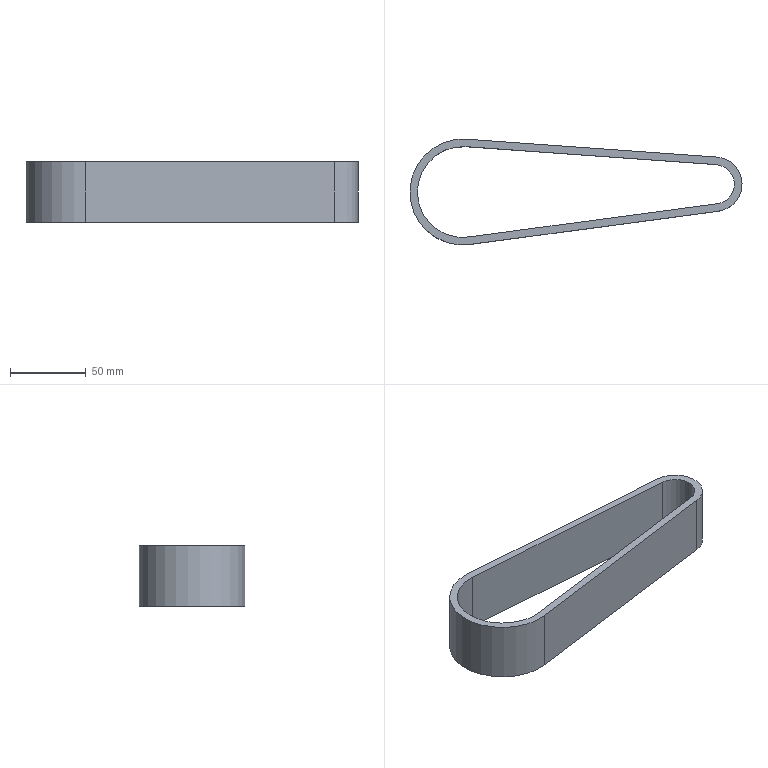Part | SolidWorks | features BaseBody 1 | 1 solid | 12 faces | box 219.551 x 70 x 40 mm | volume 97158 mm3 | cylinder 6 | plane 6 | commonest cylinder face diameters 26 x2 36 x2 60 x1 70 x1
STEP:
#1=CARTESIAN_POINT('',(-274.757,49.399,20.));
#2=VERTEX_POINT('',#1);
#3=CARTESIAN_POINT('',(-263.488,62.685,20.));
#4=VERTEX_POINT('',#3);
#5=CARTESIAN_POINT('',(-276.482,62.284,20.));
#6=DIRECTION('',(0.,0.,1.));
#7=DIRECTION('',(-0.9995,-0.03088,0.));
#8=AXIS2_PLACEMENT_3D('',#5,#6,#7);
#9=CIRCLE('',#8,13.);
#10=EDGE_CURVE('',#2,#4,#9,.T.);
#11=ORIENTED_EDGE('',*,*,#10,.T.);
#12=CARTESIAN_POINT('',(-263.488,62.685,-20.));
#13=VERTEX_POINT('',#12);
#14=CARTESIAN_POINT('',(-263.488,62.685,20.));
#15=DIRECTION('',(0.,0.,-1.));
#16=VECTOR('',#15,1000.);
#17=LINE('',#14,#16);
#18=EDGE_CURVE('',#4,#13,#17,.T.);
#19=ORIENTED_EDGE('',*,*,#18,.T.);
#20=CARTESIAN_POINT('',(-274.757,49.399,-20.));
#21=VERTEX_POINT('',#20);
#22=CARTESIAN_POINT('',(-276.482,62.284,-20.));
#23=DIRECTION('',(0.,0.,1.));
#24=DIRECTION('',(-0.9995,-0.03088,0.));
#25=AXIS2_PLACEMENT_3D('',#22,#23,#24);
#26=CIRCLE('',#25,13.);
#27=EDGE_CURVE('',#21,#13,#26,.T.);
#28=ORIENTED_EDGE('',*,*,#27,.F.);
#29=CARTESIAN_POINT('',(-274.757,49.399,20.));
#30=DIRECTION('',(0.,0.,-1.));
#31=VECTOR('',#30,1000.);
#32=LINE('',#29,#31);
#33=EDGE_CURVE('',#2,#21,#32,.T.);
#34=ORIENTED_EDGE('',*,*,#33,.F.);
#35=EDGE_LOOP('',(#11,#19,#28,#34));
#36=FACE_OUTER_BOUND('',#35,.T.);
#37=CARTESIAN_POINT('',(-276.482,62.284,20.));
#38=DIRECTION('',(0.,0.,-1.));
#39=DIRECTION('',(0.9995,0.03088,0.));
#40=AXIS2_PLACEMENT_3D('',#37,#38,#39);
#41=CYLINDRICAL_SURFACE('',#40,13.);
#42=ADVANCED_FACE('',(#36),#41,.F.);
#43=CARTESIAN_POINT('',(-258.49,62.84,20.));
#44=VERTEX_POINT('',#43);
#45=CARTESIAN_POINT('',(-275.199,80.238,20.));
#46=VERTEX_POINT('',#45);
#47=CARTESIAN_POINT('',(-276.482,62.284,20.));
#48=DIRECTION('',(0.,0.,1.));
#49=DIRECTION('',(-0.9995,-0.03088,0.));
#50=AXIS2_PLACEMENT_3D('',#47,#48,#49);
#51=CIRCLE('',#50,18.);
#52=EDGE_CURVE('',#44,#46,#51,.T.);
#53=ORIENTED_EDGE('',*,*,#52,.F.);
#54=CARTESIAN_POINT('',(-258.49,62.84,-20.));
#55=VERTEX_POINT('',#54);
#56=CARTESIAN_POINT('',(-258.49,62.84,20.));
#57=DIRECTION('',(0.,0.,-1.));
#58=VECTOR('',#57,1000.);
#59=LINE('',#56,#58);
#60=EDGE_CURVE('',#44,#55,#59,.T.);
#61=ORIENTED_EDGE('',*,*,#60,.T.);
#62=CARTESIAN_POINT('',(-275.199,80.238,-20.));
#63=VERTEX_POINT('',#62);
#64=CARTESIAN_POINT('',(-276.482,62.284,-20.));
#65=DIRECTION('',(0.,0.,1.));
#66=DIRECTION('',(-0.9995,-0.03088,0.));
#67=AXIS2_PLACEMENT_3D('',#64,#65,#66);
#68=CIRCLE('',#67,18.);
#69=EDGE_CURVE('',#55,#63,#68,.T.);
#70=ORIENTED_EDGE('',*,*,#69,.T.);
#71=CARTESIAN_POINT('',(-275.199,80.238,20.));
#72=DIRECTION('',(0.,0.,-1.));
#73=VECTOR('',#72,1000.);
#74=LINE('',#71,#73);
#75=EDGE_CURVE('',#46,#63,#74,.T.);
#76=ORIENTED_EDGE('',*,*,#75,.F.);
#77=EDGE_LOOP('',(#53,#61,#70,#76));
#78=FACE_OUTER_BOUND('',#77,.T.);
#79=CARTESIAN_POINT('',(-276.482,62.284,20.));
#80=DIRECTION('',(0.,0.,-1.));
#81=DIRECTION('',(0.9995,0.03088,0.));
#82=AXIS2_PLACEMENT_3D('',#79,#80,#81);
#83=CYLINDRICAL_SURFACE('',#82,18.);
#84=ADVANCED_FACE('',(#78),#83,.T.);
#85=CARTESIAN_POINT('',(-274.093,44.443,20.));
#86=VERTEX_POINT('',#85);
#87=CARTESIAN_POINT('',(-276.482,62.284,20.));
#88=DIRECTION('',(0.,0.,1.));
#89=DIRECTION('',(-0.9995,-0.03088,0.));
#90=AXIS2_PLACEMENT_3D('',#87,#88,#89);
#91=CIRCLE('',#90,18.);
#92=EDGE_CURVE('',#86,#44,#91,.T.);
#93=ORIENTED_EDGE('',*,*,#92,.T.);
#94=ORIENTED_EDGE('',*,*,#52,.T.);
#95=CARTESIAN_POINT('',(-440.538,92.049,20.));
#96=VERTEX_POINT('',#95);
#97=CARTESIAN_POINT('',(-275.199,80.238,20.));
#98=DIRECTION('',(-0.9975,0.07126,0.));
#99=VECTOR('',#98,1000.);
#100=LINE('',#97,#99);
#101=EDGE_CURVE('',#46,#96,#100,.T.);
#102=ORIENTED_EDGE('',*,*,#101,.T.);
#103=CARTESIAN_POINT('',(-438.388,22.448,20.));
#104=VERTEX_POINT('',#103);
#105=CARTESIAN_POINT('',(-443.032,57.138,20.));
#106=DIRECTION('',(0.,0.,1.));
#107=DIRECTION('',(-0.9995,-0.03088,0.));
#108=AXIS2_PLACEMENT_3D('',#105,#106,#107);
#109=CIRCLE('',#108,35.);
#110=EDGE_CURVE('',#96,#104,#109,.T.);
#111=ORIENTED_EDGE('',*,*,#110,.T.);
#112=CARTESIAN_POINT('',(-274.093,44.443,20.));
#113=DIRECTION('',(0.9912,0.1327,0.));
#114=VECTOR('',#113,1000.);
#115=LINE('',#112,#114);
#116=EDGE_CURVE('',#104,#86,#115,.T.);
#117=ORIENTED_EDGE('',*,*,#116,.T.);
#118=EDGE_LOOP('',(#93,#94,#102,#111,#117));
#119=FACE_OUTER_BOUND('',#118,.T.);
#120=CARTESIAN_POINT('',(-439.052,27.404,20.));
#121=VERTEX_POINT('',#120);
#122=CARTESIAN_POINT('',(-274.757,49.399,20.));
#123=DIRECTION('',(0.9912,0.1327,0.));
#124=VECTOR('',#123,1000.);
#125=LINE('',#122,#124);
#126=EDGE_CURVE('',#121,#2,#125,.T.);
#127=ORIENTED_EDGE('',*,*,#126,.F.);
#128=CARTESIAN_POINT('',(-440.895,87.062,20.));
#129=VERTEX_POINT('',#128);
#130=CARTESIAN_POINT('',(-443.032,57.138,20.));
#131=DIRECTION('',(0.,0.,1.));
#132=DIRECTION('',(-0.9995,-0.03088,0.));
#133=AXIS2_PLACEMENT_3D('',#130,#131,#132);
#134=CIRCLE('',#133,30.);
#135=EDGE_CURVE('',#129,#121,#134,.T.);
#136=ORIENTED_EDGE('',*,*,#135,.F.);
#137=CARTESIAN_POINT('',(-275.555,75.251,20.));
#138=VERTEX_POINT('',#137);
#139=CARTESIAN_POINT('',(-275.555,75.251,20.));
#140=DIRECTION('',(-0.9975,0.07126,0.));
#141=VECTOR('',#140,1000.);
#142=LINE('',#139,#141);
#143=EDGE_CURVE('',#138,#129,#142,.T.);
#144=ORIENTED_EDGE('',*,*,#143,.F.);
#145=CARTESIAN_POINT('',(-276.482,62.284,20.));
#146=DIRECTION('',(0.,0.,1.));
#147=DIRECTION('',(-0.9995,-0.03088,0.));
#148=AXIS2_PLACEMENT_3D('',#145,#146,#147);
#149=CIRCLE('',#148,13.);
#150=EDGE_CURVE('',#4,#138,#149,.T.);
#151=ORIENTED_EDGE('',*,*,#150,.F.);
#152=ORIENTED_EDGE('',*,*,#10,.F.);
#153=EDGE_LOOP('',(#127,#136,#144,#151,#152));
#154=FACE_BOUND('',#153,.T.);
#155=CARTESIAN_POINT('',(-276.482,62.284,20.));
#156=DIRECTION('',(0.,0.,1.));
#157=DIRECTION('',(-0.9995,-0.03088,0.));
#158=AXIS2_PLACEMENT_3D('',#155,#156,#157);
#159=PLANE('',#158);
#160=ADVANCED_FACE('',(#119,#154),#159,.T.);
#161=CARTESIAN_POINT('',(-274.093,44.443,-20.));
#162=VERTEX_POINT('',#161);
#163=CARTESIAN_POINT('',(-276.482,62.284,-20.));
#164=DIRECTION('',(0.,0.,1.));
#165=DIRECTION('',(-0.9995,-0.03088,0.));
#166=AXIS2_PLACEMENT_3D('',#163,#164,#165);
#167=CIRCLE('',#166,18.);
#168=EDGE_CURVE('',#162,#55,#167,.T.);
#169=ORIENTED_EDGE('',*,*,#168,.F.);
#170=CARTESIAN_POINT('',(-438.388,22.448,-20.));
#171=VERTEX_POINT('',#170);
#172=CARTESIAN_POINT('',(-274.093,44.443,-20.));
#173=DIRECTION('',(0.9912,0.1327,0.));
#174=VECTOR('',#173,1000.);
#175=LINE('',#172,#174);
#176=EDGE_CURVE('',#171,#162,#175,.T.);
#177=ORIENTED_EDGE('',*,*,#176,.F.);
#178=CARTESIAN_POINT('',(-440.538,92.049,-20.));
#179=VERTEX_POINT('',#178);
#180=CARTESIAN_POINT('',(-443.032,57.138,-20.));
#181=DIRECTION('',(0.,0.,1.));
#182=DIRECTION('',(-0.9995,-0.03088,0.));
#183=AXIS2_PLACEMENT_3D('',#180,#181,#182);
#184=CIRCLE('',#183,35.);
#185=EDGE_CURVE('',#179,#171,#184,.T.);
#186=ORIENTED_EDGE('',*,*,#185,.F.);
#187=CARTESIAN_POINT('',(-275.199,80.238,-20.));
#188=DIRECTION('',(-0.9975,0.07126,0.));
#189=VECTOR('',#188,1000.);
#190=LINE('',#187,#189);
#191=EDGE_CURVE('',#63,#179,#190,.T.);
#192=ORIENTED_EDGE('',*,*,#191,.F.);
#193=ORIENTED_EDGE('',*,*,#69,.F.);
#194=EDGE_LOOP('',(#169,#177,#186,#192,#193));
#195=FACE_OUTER_BOUND('',#194,.T.);
#196=CARTESIAN_POINT('',(-440.895,87.062,-20.));
#197=VERTEX_POINT('',#196);
#198=CARTESIAN_POINT('',(-439.052,27.404,-20.));
#199=VERTEX_POINT('',#198);
#200=CARTESIAN_POINT('',(-443.032,57.138,-20.));
#201=DIRECTION('',(0.,0.,1.));
#202=DIRECTION('',(-0.9995,-0.03088,0.));
#203=AXIS2_PLACEMENT_3D('',#200,#201,#202);
#204=CIRCLE('',#203,30.);
#205=EDGE_CURVE('',#197,#199,#204,.T.);
#206=ORIENTED_EDGE('',*,*,#205,.T.);
#207=CARTESIAN_POINT('',(-274.757,49.399,-20.));
#208=DIRECTION('',(0.9912,0.1327,0.));
#209=VECTOR('',#208,1000.);
#210=LINE('',#207,#209);
#211=EDGE_CURVE('',#199,#21,#210,.T.);
#212=ORIENTED_EDGE('',*,*,#211,.T.);
#213=ORIENTED_EDGE('',*,*,#27,.T.);
#214=CARTESIAN_POINT('',(-275.555,75.251,-20.));
#215=VERTEX_POINT('',#214);
#216=CARTESIAN_POINT('',(-276.482,62.284,-20.));
#217=DIRECTION('',(0.,0.,1.));
#218=DIRECTION('',(-0.9995,-0.03088,0.));
#219=AXIS2_PLACEMENT_3D('',#216,#217,#218);
#220=CIRCLE('',#219,13.);
#221=EDGE_CURVE('',#13,#215,#220,.T.);
#222=ORIENTED_EDGE('',*,*,#221,.T.);
#223=CARTESIAN_POINT('',(-275.555,75.251,-20.));
#224=DIRECTION('',(-0.9975,0.07126,0.));
#225=VECTOR('',#224,1000.);
#226=LINE('',#223,#225);
#227=EDGE_CURVE('',#215,#197,#226,.T.);
#228=ORIENTED_EDGE('',*,*,#227,.T.);
#229=EDGE_LOOP('',(#206,#212,#213,#222,#228));
#230=FACE_BOUND('',#229,.T.);
#231=CARTESIAN_POINT('',(-276.482,62.284,-20.));
#232=DIRECTION('',(0.,0.,1.));
#233=DIRECTION('',(-0.9995,-0.03088,0.));
#234=AXIS2_PLACEMENT_3D('',#231,#232,#233);
#235=PLANE('',#234);
#236=ADVANCED_FACE('',(#195,#230),#235,.F.);
#237=ORIENTED_EDGE('',*,*,#60,.F.);
#238=ORIENTED_EDGE('',*,*,#92,.F.);
#239=CARTESIAN_POINT('',(-274.093,44.443,20.));
#240=DIRECTION('',(0.,0.,-1.));
#241=VECTOR('',#240,1000.);
#242=LINE('',#239,#241);
#243=EDGE_CURVE('',#86,#162,#242,.T.);
#244=ORIENTED_EDGE('',*,*,#243,.T.);
#245=ORIENTED_EDGE('',*,*,#168,.T.);
#246=EDGE_LOOP('',(#237,#238,#244,#245));
#247=FACE_OUTER_BOUND('',#246,.T.);
#248=CARTESIAN_POINT('',(-276.482,62.284,20.));
#249=DIRECTION('',(0.,0.,-1.));
#250=DIRECTION('',(0.9995,0.03088,0.));
#251=AXIS2_PLACEMENT_3D('',#248,#249,#250);
#252=CYLINDRICAL_SURFACE('',#251,18.);
#253=ADVANCED_FACE('',(#247),#252,.T.);
#254=ORIENTED_EDGE('',*,*,#191,.T.);
#255=CARTESIAN_POINT('',(-440.538,92.049,20.));
#256=DIRECTION('',(0.,0.,-1.));
#257=VECTOR('',#256,1000.);
#258=LINE('',#255,#257);
#259=EDGE_CURVE('',#96,#179,#258,.T.);
#260=ORIENTED_EDGE('',*,*,#259,.F.);
#261=ORIENTED_EDGE('',*,*,#101,.F.);
#262=ORIENTED_EDGE('',*,*,#75,.T.);
#263=EDGE_LOOP('',(#254,#260,#261,#262));
#264=FACE_OUTER_BOUND('',#263,.T.);
#265=CARTESIAN_POINT('',(-275.199,80.238,20.));
#266=DIRECTION('',(-0.07126,-0.9975,0.));
#267=DIRECTION('',(0.9975,-0.07126,0.));
#268=AXIS2_PLACEMENT_3D('',#265,#266,#267);
#269=PLANE('',#268);
#270=ADVANCED_FACE('',(#264),#269,.F.);
#271=ORIENTED_EDGE('',*,*,#185,.T.);
#272=CARTESIAN_POINT('',(-438.388,22.448,20.));
#273=DIRECTION('',(0.,0.,-1.));
#274=VECTOR('',#273,1000.);
#275=LINE('',#272,#274);
#276=EDGE_CURVE('',#104,#171,#275,.T.);
#277=ORIENTED_EDGE('',*,*,#276,.F.);
#278=ORIENTED_EDGE('',*,*,#110,.F.);
#279=ORIENTED_EDGE('',*,*,#259,.T.);
#280=EDGE_LOOP('',(#271,#277,#278,#279));
#281=FACE_OUTER_BOUND('',#280,.T.);
#282=CARTESIAN_POINT('',(-443.032,57.138,20.));
#283=DIRECTION('',(0.,0.,-1.));
#284=DIRECTION('',(0.9995,0.03088,0.));
#285=AXIS2_PLACEMENT_3D('',#282,#283,#284);
#286=CYLINDRICAL_SURFACE('',#285,35.);
#287=ADVANCED_FACE('',(#281),#286,.T.);
#288=ORIENTED_EDGE('',*,*,#176,.T.);
#289=ORIENTED_EDGE('',*,*,#243,.F.);
#290=ORIENTED_EDGE('',*,*,#116,.F.);
#291=ORIENTED_EDGE('',*,*,#276,.T.);
#292=EDGE_LOOP('',(#288,#289,#290,#291));
#293=FACE_OUTER_BOUND('',#292,.T.);
#294=CARTESIAN_POINT('',(-274.093,44.443,20.));
#295=DIRECTION('',(-0.1327,0.9912,0.));
#296=DIRECTION('',(-0.9912,-0.1327,0.));
#297=AXIS2_PLACEMENT_3D('',#294,#295,#296);
#298=PLANE('',#297);
#299=ADVANCED_FACE('',(#293),#298,.F.);
#300=ORIENTED_EDGE('',*,*,#205,.F.);
#301=CARTESIAN_POINT('',(-440.895,87.062,20.));
#302=DIRECTION('',(0.,0.,-1.));
#303=VECTOR('',#302,1000.);
#304=LINE('',#301,#303);
#305=EDGE_CURVE('',#129,#197,#304,.T.);
#306=ORIENTED_EDGE('',*,*,#305,.F.);
#307=ORIENTED_EDGE('',*,*,#135,.T.);
#308=CARTESIAN_POINT('',(-439.052,27.404,20.));
#309=DIRECTION('',(0.,0.,-1.));
#310=VECTOR('',#309,1000.);
#311=LINE('',#308,#310);
#312=EDGE_CURVE('',#121,#199,#311,.T.);
#313=ORIENTED_EDGE('',*,*,#312,.T.);
#314=EDGE_LOOP('',(#300,#306,#307,#313));
#315=FACE_OUTER_BOUND('',#314,.T.);
#316=CARTESIAN_POINT('',(-443.032,57.138,20.));
#317=DIRECTION('',(0.,0.,-1.));
#318=DIRECTION('',(0.9995,0.03088,0.));
#319=AXIS2_PLACEMENT_3D('',#316,#317,#318);
#320=CYLINDRICAL_SURFACE('',#319,30.);
#321=ADVANCED_FACE('',(#315),#320,.F.);
#322=ORIENTED_EDGE('',*,*,#211,.F.);
#323=ORIENTED_EDGE('',*,*,#312,.F.);
#324=ORIENTED_EDGE('',*,*,#126,.T.);
#325=ORIENTED_EDGE('',*,*,#33,.T.);
#326=EDGE_LOOP('',(#322,#323,#324,#325));
#327=FACE_OUTER_BOUND('',#326,.T.);
#328=CARTESIAN_POINT('',(-274.757,49.399,20.));
#329=DIRECTION('',(-0.1327,0.9912,0.));
#330=DIRECTION('',(-0.9912,-0.1327,0.));
#331=AXIS2_PLACEMENT_3D('',#328,#329,#330);
#332=PLANE('',#331);
#333=ADVANCED_FACE('',(#327),#332,.T.);
#334=ORIENTED_EDGE('',*,*,#18,.F.);
#335=ORIENTED_EDGE('',*,*,#150,.T.);
#336=CARTESIAN_POINT('',(-275.555,75.251,20.));
#337=DIRECTION('',(0.,0.,-1.));
#338=VECTOR('',#337,1000.);
#339=LINE('',#336,#338);
#340=EDGE_CURVE('',#138,#215,#339,.T.);
#341=ORIENTED_EDGE('',*,*,#340,.T.);
#342=ORIENTED_EDGE('',*,*,#221,.F.);
#343=EDGE_LOOP('',(#334,#335,#341,#342));
#344=FACE_OUTER_BOUND('',#343,.T.);
#345=CARTESIAN_POINT('',(-276.482,62.284,20.));
#346=DIRECTION('',(0.,0.,-1.));
#347=DIRECTION('',(0.9995,0.03088,0.));
#348=AXIS2_PLACEMENT_3D('',#345,#346,#347);
#349=CYLINDRICAL_SURFACE('',#348,13.);
#350=ADVANCED_FACE('',(#344),#349,.F.);
#351=ORIENTED_EDGE('',*,*,#227,.F.);
#352=ORIENTED_EDGE('',*,*,#340,.F.);
#353=ORIENTED_EDGE('',*,*,#143,.T.);
#354=ORIENTED_EDGE('',*,*,#305,.T.);
#355=EDGE_LOOP('',(#351,#352,#353,#354));
#356=FACE_OUTER_BOUND('',#355,.T.);
#357=CARTESIAN_POINT('',(-275.555,75.251,20.));
#358=DIRECTION('',(-0.07126,-0.9975,0.));
#359=DIRECTION('',(0.9975,-0.07126,0.));
#360=AXIS2_PLACEMENT_3D('',#357,#358,#359);
#361=PLANE('',#360);
#362=ADVANCED_FACE('',(#356),#361,.T.);
#363=CLOSED_SHELL('',(#42,#84,#160,#236,#253,#270,#287,#299,#321,#333,#350,#362));
#364=MANIFOLD_SOLID_BREP('',#363);
#365=CARTESIAN_POINT('',(0.,0.,0.));
#366=DIRECTION('',(0.,0.,1.));
#367=DIRECTION('',(1.,0.,0.));
#368=AXIS2_PLACEMENT_3D('',#365,#366,#367);
#369=(LENGTH_UNIT()NAMED_UNIT(*)SI_UNIT(.MILLI.,.METRE.));
#370=UNCERTAINTY_MEASURE_WITH_UNIT(LENGTH_MEASURE(0.00001),#369,'','');
#371=(NAMED_UNIT(*)PLANE_ANGLE_UNIT()SI_UNIT($,.RADIAN.));
#372=(NAMED_UNIT(*)SI_UNIT($,.STERADIAN.)SOLID_ANGLE_UNIT());
#373=(GEOMETRIC_REPRESENTATION_CONTEXT(3)GLOBAL_UNCERTAINTY_ASSIGNED_CONTEXT((#370))GLOBAL_UNIT_ASSIGNED_CONTEXT((#369,#371,#372))REPRESENTATION_CONTEXT('',''));
#374=ADVANCED_BREP_SHAPE_REPRESENTATION('',(#364,#368),#373);